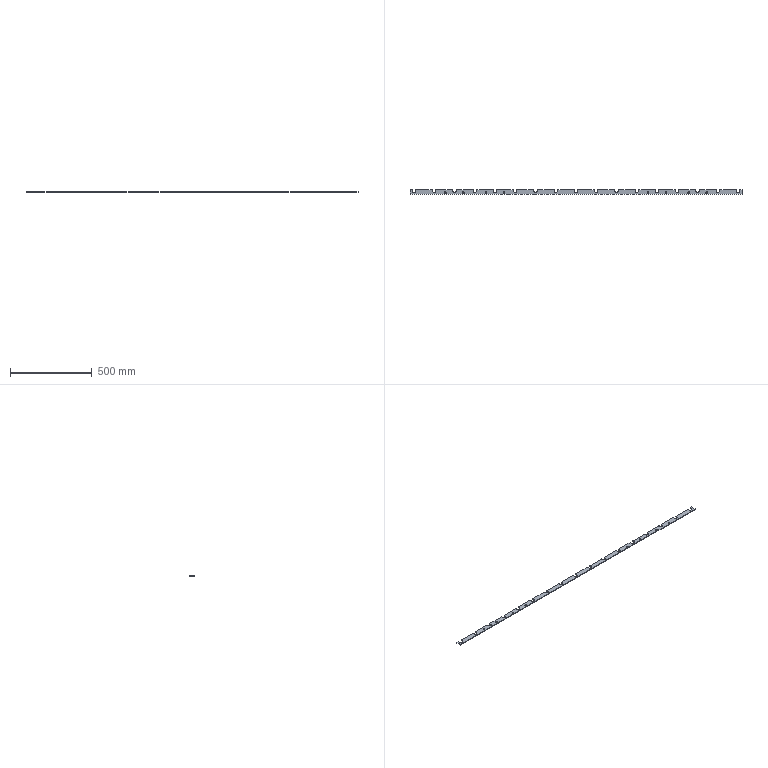Part | SolidWorks | features ICE 2, Extrusion 1, Fillet 1 | 1 solid | 124 faces | box 2030 x 30 x 4 mm | volume 216015 mm3 | cylinder 67 | plane 57 | commonest cylinder face diameters 6 x34 20 x17 11 x16